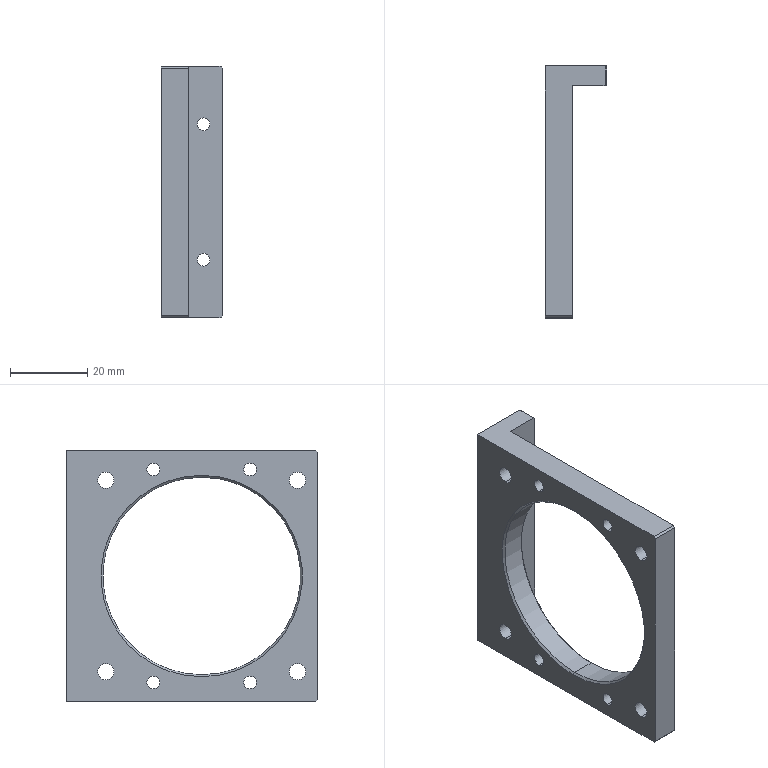Part | STEP file | 1 solid | 38 faces | box 16 x 65 x 65 mm | volume 17444 mm3 | cylinder 22 | plane 12 | cone 4 | commonest cylinder face diameters 3.3 x12 4.2 x8 51 x2